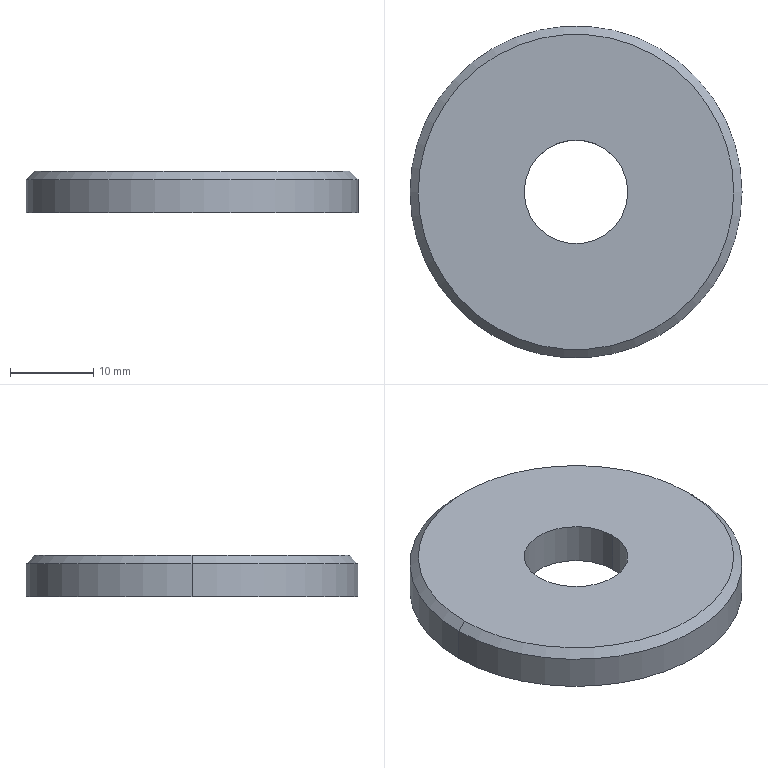Part | SolidWorks | features Chamfer 1, Extrusion 1 | 1 solid | 8 faces | box 40 x 40 x 5 mm | volume 5608 mm3 | cylinder 4 | cone 2 | plane 2 | commonest cylinder face diameters 12.5 x2 40 x2
STEP:
#1=CARTESIAN_POINT('',(19.,0.,5.));
#2=VERTEX_POINT('',#1);
#3=CARTESIAN_POINT('',(-19.,0.,5.));
#4=VERTEX_POINT('',#3);
#5=CARTESIAN_POINT('',(0.,0.,5.));
#6=DIRECTION('',(0.,0.,1.));
#7=DIRECTION('',(1.,0.,0.));
#8=AXIS2_PLACEMENT_3D('',#5,#6,#7);
#9=CIRCLE('',#8,19.);
#10=EDGE_CURVE('',#2,#4,#9,.T.);
#11=ORIENTED_EDGE('',*,*,#10,.F.);
#12=CARTESIAN_POINT('',(20.,0.,4.));
#13=VERTEX_POINT('',#12);
#14=CARTESIAN_POINT('',(19.,0.,5.));
#15=DIRECTION('',(0.7071,0.,-0.7071));
#16=VECTOR('',#15,1000.);
#17=LINE('',#14,#16);
#18=EDGE_CURVE('',#2,#13,#17,.T.);
#19=ORIENTED_EDGE('',*,*,#18,.T.);
#20=CARTESIAN_POINT('',(-20.,0.,4.));
#21=VERTEX_POINT('',#20);
#22=CARTESIAN_POINT('',(0.,0.,4.));
#23=DIRECTION('',(0.,0.,-1.));
#24=DIRECTION('',(1.,0.,0.));
#25=AXIS2_PLACEMENT_3D('',#22,#23,#24);
#26=CIRCLE('',#25,20.);
#27=EDGE_CURVE('',#21,#13,#26,.T.);
#28=ORIENTED_EDGE('',*,*,#27,.F.);
#29=CARTESIAN_POINT('',(-19.,0.,5.));
#30=DIRECTION('',(-0.7071,0.,-0.7071));
#31=VECTOR('',#30,1000.);
#32=LINE('',#29,#31);
#33=EDGE_CURVE('',#4,#21,#32,.T.);
#34=ORIENTED_EDGE('',*,*,#33,.F.);
#35=EDGE_LOOP('',(#11,#19,#28,#34));
#36=FACE_OUTER_BOUND('',#35,.T.);
#37=CARTESIAN_POINT('',(0.,0.,5.));
#38=DIRECTION('',(0.,0.,-1.));
#39=DIRECTION('',(-1.,0.,0.));
#40=AXIS2_PLACEMENT_3D('',#37,#38,#39);
#41=CONICAL_SURFACE('',#40,19.,0.7854);
#42=ADVANCED_FACE('',(#36),#41,.T.);
#43=CARTESIAN_POINT('',(-6.25,0.,5.));
#44=VERTEX_POINT('',#43);
#45=CARTESIAN_POINT('',(6.25,0.,5.));
#46=VERTEX_POINT('',#45);
#47=CARTESIAN_POINT('',(0.,0.,5.));
#48=DIRECTION('',(0.,0.,1.));
#49=DIRECTION('',(1.,0.,0.));
#50=AXIS2_PLACEMENT_3D('',#47,#48,#49);
#51=CIRCLE('',#50,6.25);
#52=EDGE_CURVE('',#44,#46,#51,.T.);
#53=ORIENTED_EDGE('',*,*,#52,.T.);
#54=CARTESIAN_POINT('',(6.25,0.,0.));
#55=VERTEX_POINT('',#54);
#56=CARTESIAN_POINT('',(6.25,0.,5.));
#57=DIRECTION('',(0.,0.,-1.));
#58=VECTOR('',#57,1000.);
#59=LINE('',#56,#58);
#60=EDGE_CURVE('',#46,#55,#59,.T.);
#61=ORIENTED_EDGE('',*,*,#60,.T.);
#62=CARTESIAN_POINT('',(-6.25,0.,0.));
#63=VERTEX_POINT('',#62);
#64=CARTESIAN_POINT('',(0.,0.,0.));
#65=DIRECTION('',(0.,0.,1.));
#66=DIRECTION('',(1.,0.,0.));
#67=AXIS2_PLACEMENT_3D('',#64,#65,#66);
#68=CIRCLE('',#67,6.25);
#69=EDGE_CURVE('',#63,#55,#68,.T.);
#70=ORIENTED_EDGE('',*,*,#69,.F.);
#71=CARTESIAN_POINT('',(-6.25,0.,5.));
#72=DIRECTION('',(0.,0.,-1.));
#73=VECTOR('',#72,1000.);
#74=LINE('',#71,#73);
#75=EDGE_CURVE('',#44,#63,#74,.T.);
#76=ORIENTED_EDGE('',*,*,#75,.F.);
#77=EDGE_LOOP('',(#53,#61,#70,#76));
#78=FACE_OUTER_BOUND('',#77,.T.);
#79=CARTESIAN_POINT('',(0.,0.,5.));
#80=DIRECTION('',(0.,0.,-1.));
#81=DIRECTION('',(-1.,0.,0.));
#82=AXIS2_PLACEMENT_3D('',#79,#80,#81);
#83=CYLINDRICAL_SURFACE('',#82,6.25);
#84=ADVANCED_FACE('',(#78),#83,.F.);
#85=ORIENTED_EDGE('',*,*,#27,.T.);
#86=CARTESIAN_POINT('',(20.,0.,0.));
#87=VERTEX_POINT('',#86);
#88=CARTESIAN_POINT('',(20.,0.,5.));
#89=DIRECTION('',(0.,0.,-1.));
#90=VECTOR('',#89,1000.);
#91=LINE('',#88,#90);
#92=EDGE_CURVE('',#13,#87,#91,.T.);
#93=ORIENTED_EDGE('',*,*,#92,.T.);
#94=CARTESIAN_POINT('',(-20.,0.,0.));
#95=VERTEX_POINT('',#94);
#96=CARTESIAN_POINT('',(0.,0.,0.));
#97=DIRECTION('',(0.,0.,1.));
#98=DIRECTION('',(1.,0.,0.));
#99=AXIS2_PLACEMENT_3D('',#96,#97,#98);
#100=CIRCLE('',#99,20.);
#101=EDGE_CURVE('',#87,#95,#100,.T.);
#102=ORIENTED_EDGE('',*,*,#101,.T.);
#103=CARTESIAN_POINT('',(-20.,0.,5.));
#104=DIRECTION('',(0.,0.,-1.));
#105=VECTOR('',#104,1000.);
#106=LINE('',#103,#105);
#107=EDGE_CURVE('',#21,#95,#106,.T.);
#108=ORIENTED_EDGE('',*,*,#107,.F.);
#109=EDGE_LOOP('',(#85,#93,#102,#108));
#110=FACE_OUTER_BOUND('',#109,.T.);
#111=CARTESIAN_POINT('',(0.,0.,5.));
#112=DIRECTION('',(0.,0.,-1.));
#113=DIRECTION('',(-1.,0.,0.));
#114=AXIS2_PLACEMENT_3D('',#111,#112,#113);
#115=CYLINDRICAL_SURFACE('',#114,20.);
#116=ADVANCED_FACE('',(#110),#115,.T.);
#117=CARTESIAN_POINT('',(0.,0.,5.));
#118=DIRECTION('',(0.,0.,1.));
#119=DIRECTION('',(1.,0.,0.));
#120=AXIS2_PLACEMENT_3D('',#117,#118,#119);
#121=CIRCLE('',#120,19.);
#122=EDGE_CURVE('',#4,#2,#121,.T.);
#123=ORIENTED_EDGE('',*,*,#122,.T.);
#124=ORIENTED_EDGE('',*,*,#10,.T.);
#125=EDGE_LOOP('',(#123,#124));
#126=FACE_OUTER_BOUND('',#125,.T.);
#127=ORIENTED_EDGE('',*,*,#52,.F.);
#128=CARTESIAN_POINT('',(0.,0.,5.));
#129=DIRECTION('',(0.,0.,1.));
#130=DIRECTION('',(1.,0.,0.));
#131=AXIS2_PLACEMENT_3D('',#128,#129,#130);
#132=CIRCLE('',#131,6.25);
#133=EDGE_CURVE('',#46,#44,#132,.T.);
#134=ORIENTED_EDGE('',*,*,#133,.F.);
#135=EDGE_LOOP('',(#127,#134));
#136=FACE_BOUND('',#135,.T.);
#137=CARTESIAN_POINT('',(0.,0.,5.));
#138=DIRECTION('',(0.,0.,1.));
#139=DIRECTION('',(1.,0.,0.));
#140=AXIS2_PLACEMENT_3D('',#137,#138,#139);
#141=PLANE('',#140);
#142=ADVANCED_FACE('',(#126,#136),#141,.T.);
#143=CARTESIAN_POINT('',(0.,0.,0.));
#144=DIRECTION('',(0.,0.,1.));
#145=DIRECTION('',(1.,0.,0.));
#146=AXIS2_PLACEMENT_3D('',#143,#144,#145);
#147=CIRCLE('',#146,20.);
#148=EDGE_CURVE('',#95,#87,#147,.T.);
#149=ORIENTED_EDGE('',*,*,#148,.F.);
#150=ORIENTED_EDGE('',*,*,#101,.F.);
#151=EDGE_LOOP('',(#149,#150));
#152=FACE_OUTER_BOUND('',#151,.T.);
#153=ORIENTED_EDGE('',*,*,#69,.T.);
#154=CARTESIAN_POINT('',(0.,0.,0.));
#155=DIRECTION('',(0.,0.,1.));
#156=DIRECTION('',(1.,0.,0.));
#157=AXIS2_PLACEMENT_3D('',#154,#155,#156);
#158=CIRCLE('',#157,6.25);
#159=EDGE_CURVE('',#55,#63,#158,.T.);
#160=ORIENTED_EDGE('',*,*,#159,.T.);
#161=EDGE_LOOP('',(#153,#160));
#162=FACE_BOUND('',#161,.T.);
#163=CARTESIAN_POINT('',(0.,0.,0.));
#164=DIRECTION('',(0.,0.,1.));
#165=DIRECTION('',(1.,0.,0.));
#166=AXIS2_PLACEMENT_3D('',#163,#164,#165);
#167=PLANE('',#166);
#168=ADVANCED_FACE('',(#152,#162),#167,.F.);
#169=ORIENTED_EDGE('',*,*,#92,.F.);
#170=CARTESIAN_POINT('',(0.,0.,4.));
#171=DIRECTION('',(0.,0.,-1.));
#172=DIRECTION('',(1.,0.,0.));
#173=AXIS2_PLACEMENT_3D('',#170,#171,#172);
#174=CIRCLE('',#173,20.);
#175=EDGE_CURVE('',#13,#21,#174,.T.);
#176=ORIENTED_EDGE('',*,*,#175,.T.);
#177=ORIENTED_EDGE('',*,*,#107,.T.);
#178=ORIENTED_EDGE('',*,*,#148,.T.);
#179=EDGE_LOOP('',(#169,#176,#177,#178));
#180=FACE_OUTER_BOUND('',#179,.T.);
#181=CARTESIAN_POINT('',(0.,0.,5.));
#182=DIRECTION('',(0.,0.,-1.));
#183=DIRECTION('',(-1.,0.,0.));
#184=AXIS2_PLACEMENT_3D('',#181,#182,#183);
#185=CYLINDRICAL_SURFACE('',#184,20.);
#186=ADVANCED_FACE('',(#180),#185,.T.);
#187=ORIENTED_EDGE('',*,*,#60,.F.);
#188=ORIENTED_EDGE('',*,*,#133,.T.);
#189=ORIENTED_EDGE('',*,*,#75,.T.);
#190=ORIENTED_EDGE('',*,*,#159,.F.);
#191=EDGE_LOOP('',(#187,#188,#189,#190));
#192=FACE_OUTER_BOUND('',#191,.T.);
#193=CARTESIAN_POINT('',(0.,0.,5.));
#194=DIRECTION('',(0.,0.,-1.));
#195=DIRECTION('',(-1.,0.,0.));
#196=AXIS2_PLACEMENT_3D('',#193,#194,#195);
#197=CYLINDRICAL_SURFACE('',#196,6.25);
#198=ADVANCED_FACE('',(#192),#197,.F.);
#199=ORIENTED_EDGE('',*,*,#18,.F.);
#200=ORIENTED_EDGE('',*,*,#122,.F.);
#201=ORIENTED_EDGE('',*,*,#33,.T.);
#202=ORIENTED_EDGE('',*,*,#175,.F.);
#203=EDGE_LOOP('',(#199,#200,#201,#202));
#204=FACE_OUTER_BOUND('',#203,.T.);
#205=CARTESIAN_POINT('',(0.,0.,5.));
#206=DIRECTION('',(0.,0.,-1.));
#207=DIRECTION('',(-1.,0.,0.));
#208=AXIS2_PLACEMENT_3D('',#205,#206,#207);
#209=CONICAL_SURFACE('',#208,19.,0.7854);
#210=ADVANCED_FACE('',(#204),#209,.T.);
#211=CLOSED_SHELL('',(#42,#84,#116,#142,#168,#186,#198,#210));
#212=MANIFOLD_SOLID_BREP('',#211);
#213=CARTESIAN_POINT('',(0.,0.,0.));
#214=DIRECTION('',(0.,0.,1.));
#215=DIRECTION('',(1.,0.,0.));
#216=AXIS2_PLACEMENT_3D('',#213,#214,#215);
#217=(LENGTH_UNIT()NAMED_UNIT(*)SI_UNIT(.MILLI.,.METRE.));
#218=UNCERTAINTY_MEASURE_WITH_UNIT(LENGTH_MEASURE(0.00001),#217,'','');
#219=(NAMED_UNIT(*)PLANE_ANGLE_UNIT()SI_UNIT($,.RADIAN.));
#220=(NAMED_UNIT(*)SI_UNIT($,.STERADIAN.)SOLID_ANGLE_UNIT());
#221=(GEOMETRIC_REPRESENTATION_CONTEXT(3)GLOBAL_UNCERTAINTY_ASSIGNED_CONTEXT((#218))GLOBAL_UNIT_ASSIGNED_CONTEXT((#217,#219,#220))REPRESENTATION_CONTEXT('',''));
#222=ADVANCED_BREP_SHAPE_REPRESENTATION('',(#212,#216),#221);